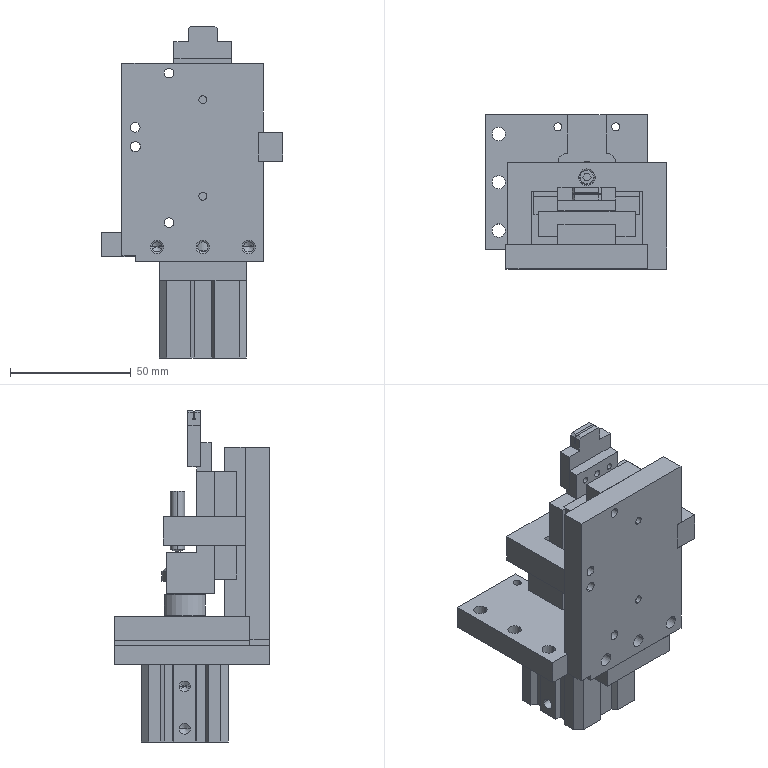Part | NX | 10 solids | 396 faces | box 75 x 64 x 137.498 mm | volume 195106 mm3 | plane 166 | cylinder 157 | cone 72 | sphere 1 | commonest cylinder face diameters 4.2 x18 4.5 x16 5.5 x16 9 x16 2.5 x12 3.3 x12